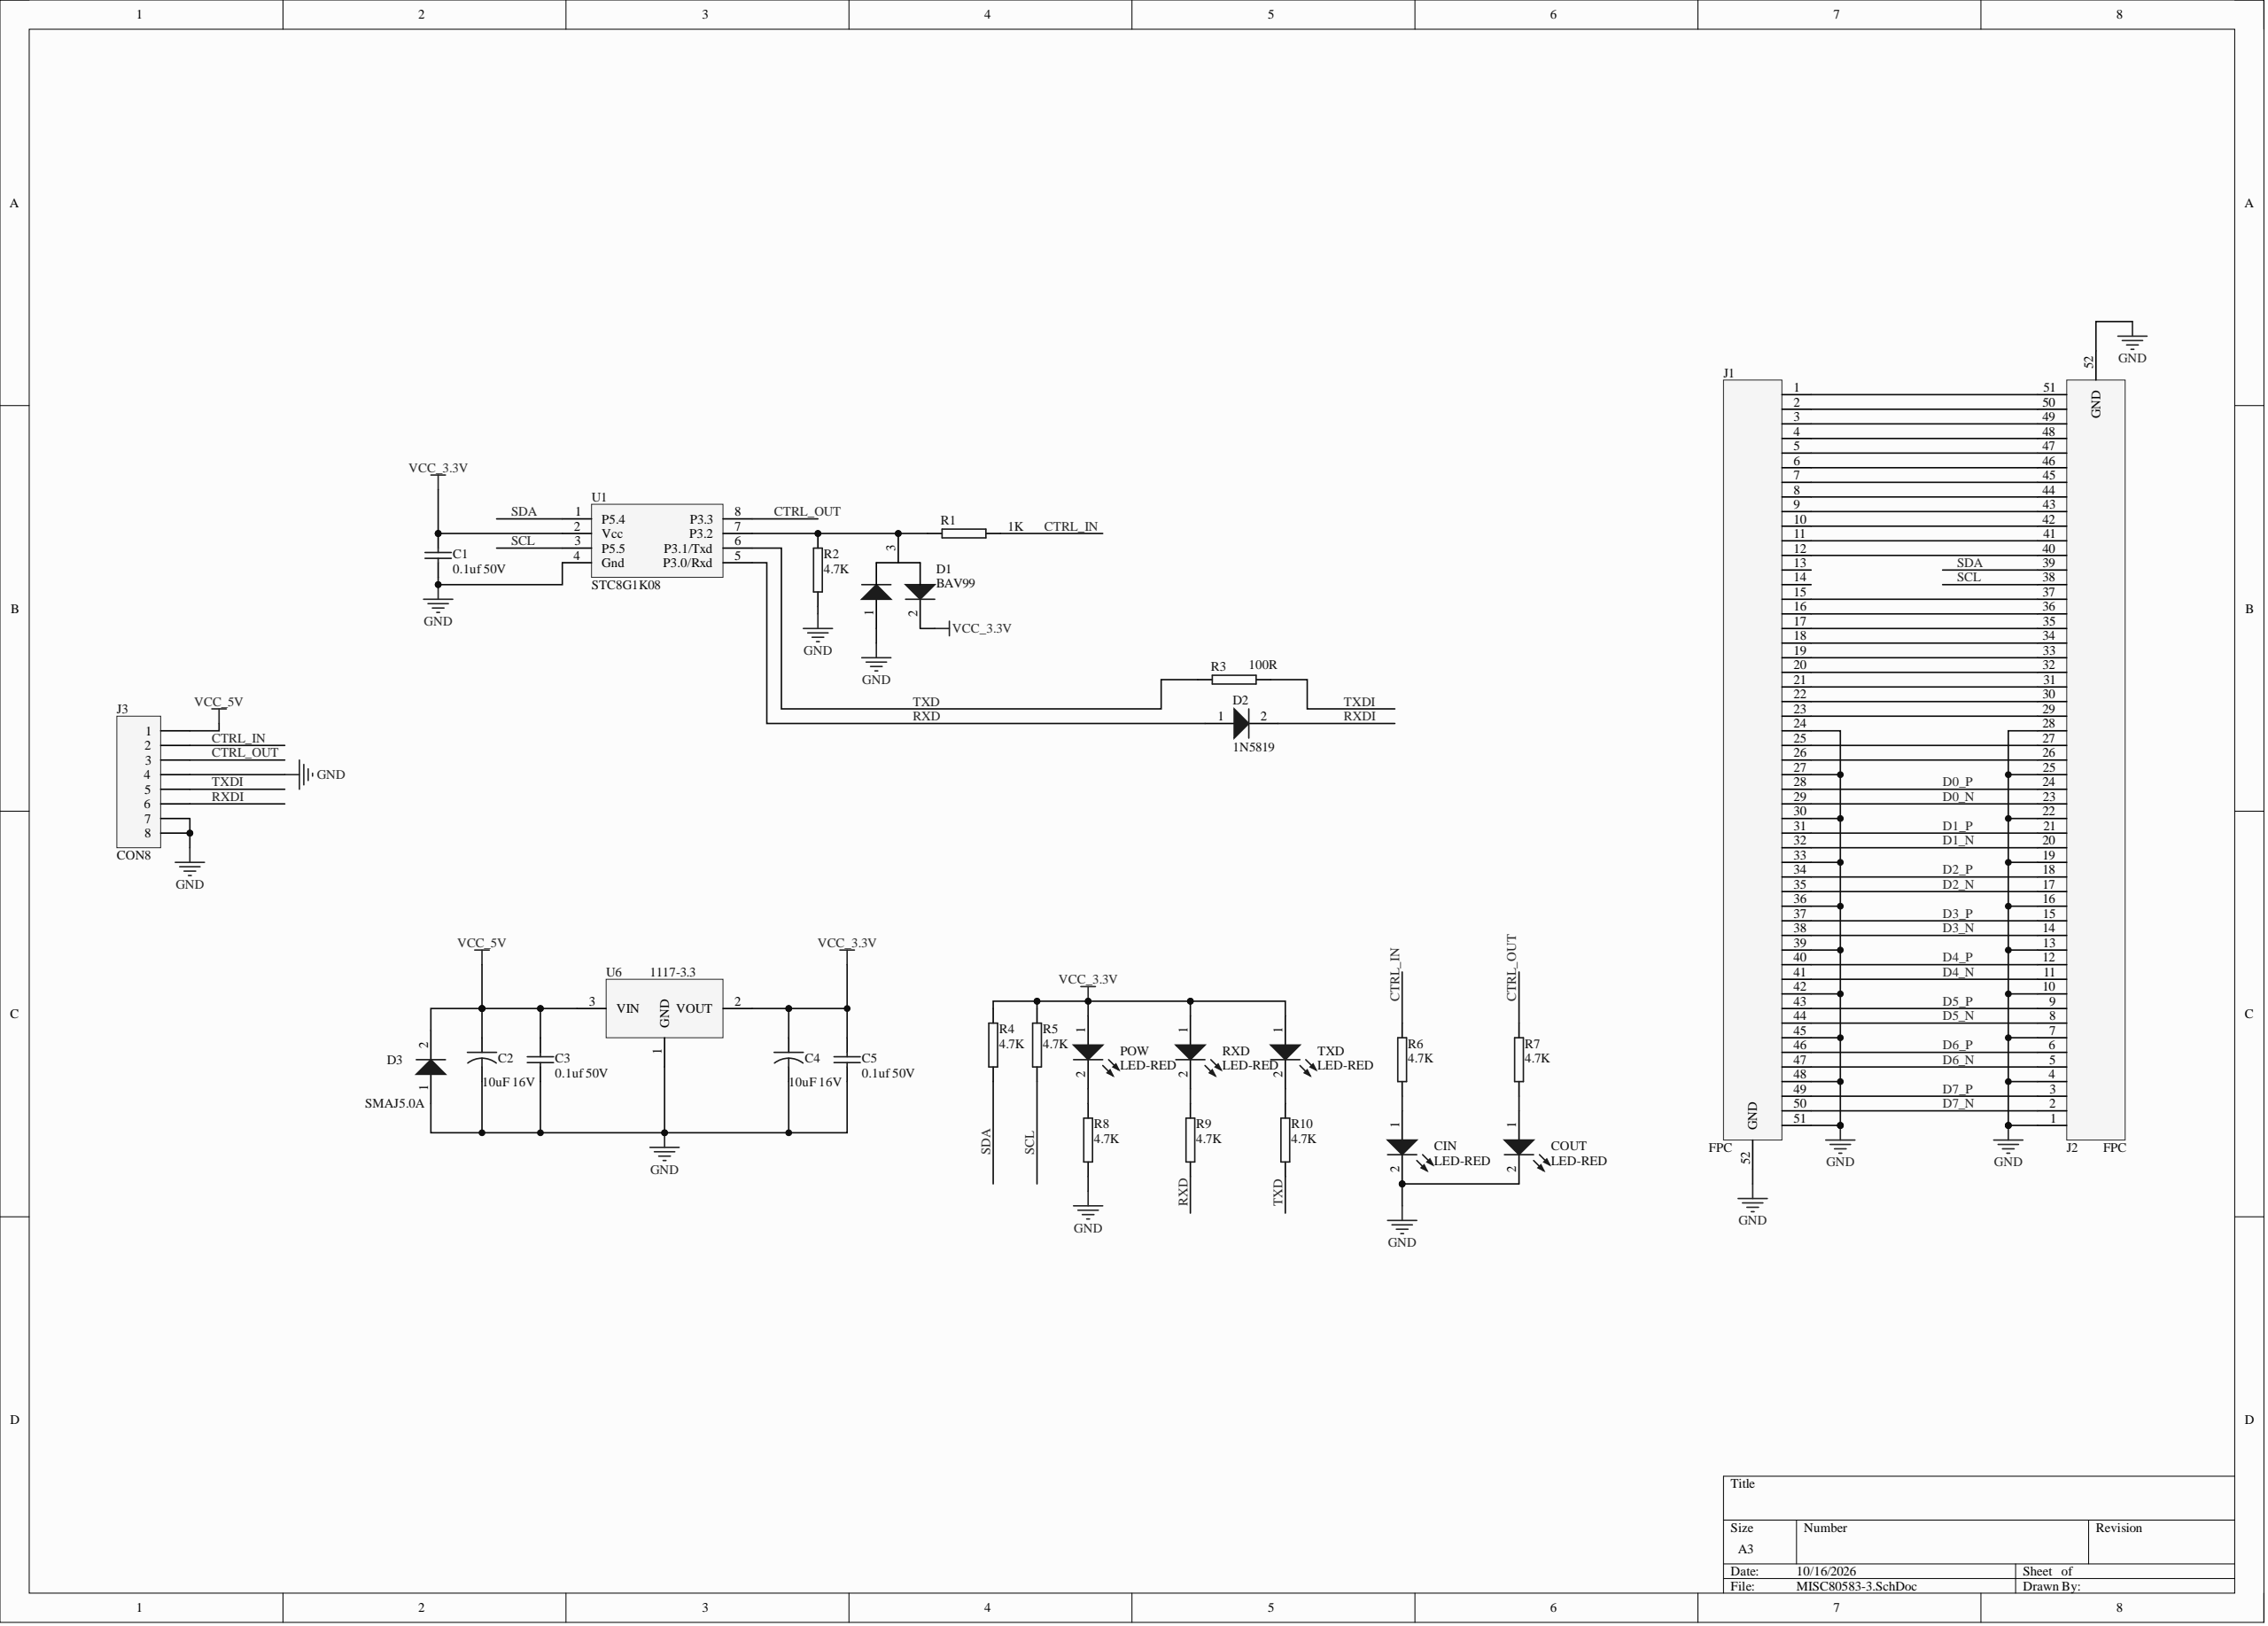Circuit board | Altium Designer | 28 parts | 56 nets
Bill of materials:
Comment,Description,Designator,Footprint,LibRef,Quantity
"0.1uf 50V","Capacitor","C1, C3, C5","0603C","CAP","3"
"10uF 16V","Capacitor","C2, C4","0805C","CAPACITOR","2"
"LED-RED","Typical RED, GREEN, YELLOW, AMBER GaAs LED","CIN, COUT, POW, RXD, TXD","LED0603","LED2","5"
"BAV99","","D1","SOT-23","BAV99","1"
"1N5819","","D2","SOD-323","1N5819","1"
"SMAJ5.0A","","D3","1N5822","1N5819","1"
"FPC","","J1, J2","FPC-0.5-51P","FPC-0.5-51P","2"
"CON8","Connector","J3","CON6-Lay","CON8","1"
"1K","","R1","0603R","RES2","1"
"4.7K","","R2, R4, R5, R6, R7, R8, R9, R10","0603R","RES2","8"
"100R","","R3","0603R","RES2","1"
"STC8G1K08","","U1","so-8","STC8G1K08","1"
"1117-3.3","","U6","SOT-223","AS1117","1"
Netlist (Protel format):
[
C1
0603C
0.1uf 50V



]
[
C2
0805C
10uF 16V



]
[
C3
0603C
0.1uf 50V



]
[
C4
0805C
10uF 16V



]
[
C5
0603C
0.1uf 50V



]
[
CIN
LED0603
LED-RED



]
[
COUT
LED0603
LED-RED



]
[
D1
SOT-23
BAV99



]
[
D2
SOD-323
1N5819



]
[
D3
1N5822
SMAJ5.0A



]
[
J1
FPC-0.5-51P
FPC



]
[
J2
FPC-0.5-51P
FPC



]
[
J3
CON6-Lay
CON8



]
[
POW
LED0603
LED-RED



]
[
R1
0603R
1K



]
[
R2
0603R
4.7K



]
[
R3
0603R
100R



]
[
R4
0603R
4.7K



]
[
R5
0603R
4.7K



]
[
R6
0603R
4.7K



]
[
R7
0603R
4.7K



]
[
R8
0603R
4.7K



]
[
R9
0603R
4.7K



]
[
R10
0603R
4.7K



]
[
RXD
LED0603
LED-RED



]
[
TXD
LED0603
LED-RED



]
[
U1
so-8
STC8G1K08



]
[
U6
SOT-223
1117-3.3



]
(
VCC_5V
C2-1
C3-1
D3-2
J3-1
U6-3
)
(
VCC_3.3V
C1-2
C4-1
C5-1
D1-2
POW-1
R4-2
R5-2
RXD-1
TXD-1
U1-2
U6-2
)
(
TXDI
J3-5
R3-2
)
(
TXD
R3-1
R10-1
U1-6
)
(
SDA
J2-39
R4-1
U1-1
)
(
SCL
J2-38
R5-1
U1-3
)
(
RXDI
D2-2
J3-6
)
(
RXD
D2-1
R9-1
U1-5
)
(
NetR10_2
R10-2
TXD-2
)
(
NetR9_2
R9-2
RXD-2
)
(
NetPOW_2
POW-2
R8-2
)
(
NetJ1_26
J1-26
J2-26
)
(
NetJ1_25
J1-25
J2-27
)
(
NetJ1_23
J1-23
J2-29
)
(
NetJ1_22
J1-22
J2-30
)
(
NetJ1_21
J1-21
J2-31
)
(
NetJ1_20
J1-20
J2-32
)
(
NetJ1_19
J1-19
J2-33
)
(
NetJ1_18
J1-18
J2-34
)
(
NetJ1_17
J1-17
J2-35
)
(
NetJ1_16
J1-16
J2-36
)
(
NetJ1_15
J1-15
J2-37
)
(
NetJ1_12
J1-12
J2-40
)
(
NetJ1_11
J1-11
J2-41
)
(
NetJ1_10
J1-10
J2-42
)
(
NetJ1_9
J1-9
J2-43
)
(
NetJ1_8
J1-8
J2-44
)
(
NetJ1_7
J1-7
J2-45
)
(
NetJ1_6
J1-6
J2-46
)
(
NetJ1_5
J1-5
J2-47
)
(
NetJ1_4
J1-4
J2-48
)
(
NetJ1_3
J1-3
J2-49
)
(
NetJ1_2
J1-2
J2-50
)
(
NetJ1_1
J1-1
J2-51
)
(
NetD1_3
D1-3
R1-1
R2-2
U1-7
)
(
NetCOUT_1
COUT-1
R7-1
)
(
NetCIN_1
CIN-1
R6-1
)
(
GND
C1-1
C2-2
C3-2
C4-2
C5-2
CIN-2
COUT-2
D1-1
D3-1
J1-24
J1-27
J1-30
J1-33
J1-36
J1-39
J1-42
J1-45
J1-48
J1-51
J1-52
J2-1
J2-4
J2-7
J2-10
J2-13
J2-16
J2-19
J2-22
J2-25
J2-28
J2-52
J3-4
J3-7
J3-8
R2-1
R8-1
U1-4
U6-1
)
(
D7_P
J1-49
J2-3
)
(
D7_N
J1-50
J2-2
)
(
D6_P
J1-46
J2-6
)
(
D6_N
J1-47
J2-5
)
(
D5_P
J1-43
J2-9
)
(
D5_N
J1-44
J2-8
)
(
D4_P
J1-40
J2-12
)
(
D4_N
J1-41
J2-11
)
(
D3_P
J1-37
J2-15
)
(
D3_N
J1-38
J2-14
)
(
D2_P
J1-34
J2-18
)
(
D2_N
J1-35
J2-17
)
(
D1_P
J1-31
J2-21
)
(
D1_N
J1-32
J2-20
)
(
D0_P
J1-28
J2-24
)
(
D0_N
J1-29
J2-23
)
(
CTRL_OUT
J3-3
R7-2
U1-8
)
(
CTRL_IN
J3-2
R1-2
R6-2
)